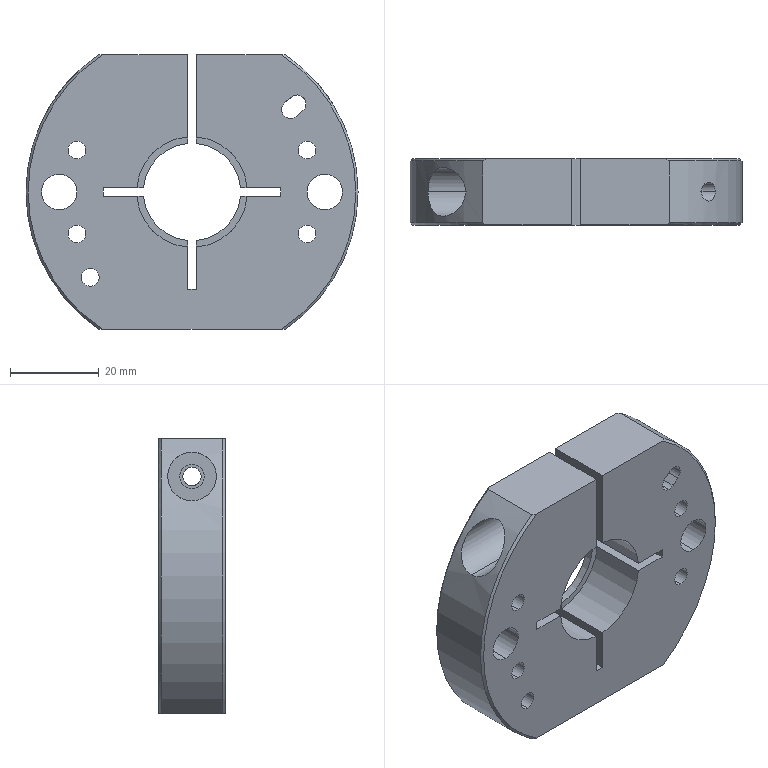Part | SolidWorks | features ICE 12, 3DProfileFeature 2, HoleWzd 2, Chamfer 1, CirPattern 1, Extrusion 1 | 1 solid | 88 faces | box 75 x 15 x 62 mm | volume 46080 mm3 | cylinder 49 | plane 27 | cone 12 | commonest cylinder face diameters 4 x13 8 x12 2.5 x8 22 x4 25 x4 4.2 x2